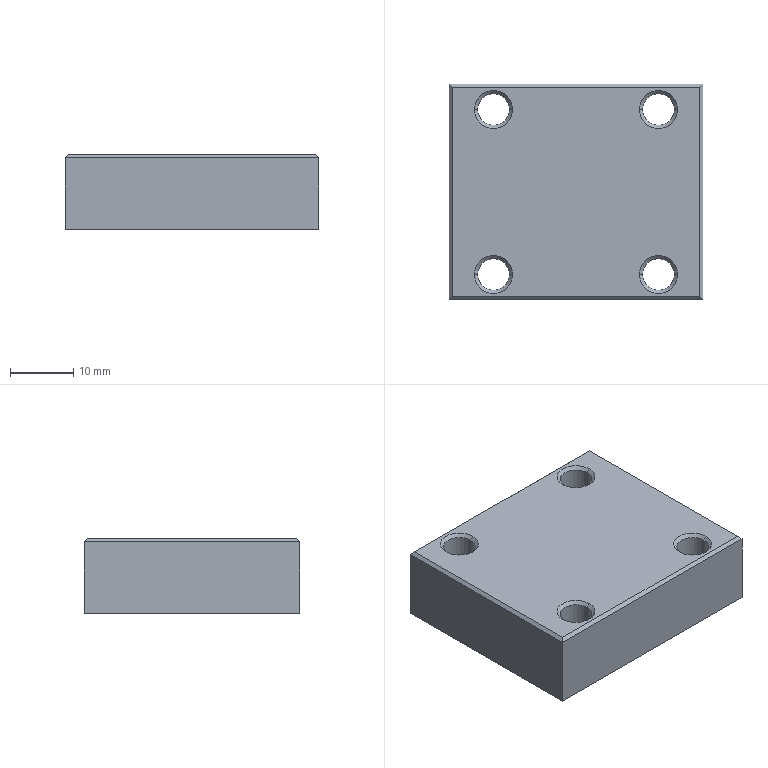Part | NX | 1 solid | 26 faces | box 40 x 34 x 11.83 mm | volume 15133 mm3 | plane 10 | cylinder 8 | cone 8 | commonest cylinder face diameters 5 x8
STEP:
#1=CARTESIAN_POINT('',(0.,0.,8.07));
#2=VERTEX_POINT('',#1);
#3=CARTESIAN_POINT('',(0.,-34.,8.07));
#4=VERTEX_POINT('',#3);
#5=CARTESIAN_POINT('',(0.,0.,8.07));
#6=DIRECTION('',(0.,-1.,0.));
#7=VECTOR('',#6,1000.);
#8=LINE('',#5,#7);
#9=EDGE_CURVE('',#2,#4,#8,.T.);
#10=ORIENTED_EDGE('',*,*,#9,.T.);
#11=CARTESIAN_POINT('',(0.5,-33.5,8.57));
#12=VERTEX_POINT('',#11);
#13=CARTESIAN_POINT('',(-8.07,-42.07,0.));
#14=DIRECTION('',(-0.5774,-0.5774,-0.5774));
#15=VECTOR('',#14,1000.);
#16=LINE('',#13,#15);
#17=EDGE_CURVE('',#12,#4,#16,.T.);
#18=ORIENTED_EDGE('',*,*,#17,.F.);
#19=CARTESIAN_POINT('',(0.5,-0.5,8.57));
#20=VERTEX_POINT('',#19);
#21=CARTESIAN_POINT('',(0.5,0.,8.57));
#22=DIRECTION('',(0.,1.,0.));
#23=VECTOR('',#22,1000.);
#24=LINE('',#21,#23);
#25=EDGE_CURVE('',#12,#20,#24,.T.);
#26=ORIENTED_EDGE('',*,*,#25,.T.);
#27=CARTESIAN_POINT('',(-8.07,8.07,0.));
#28=DIRECTION('',(-0.5774,0.5774,-0.5774));
#29=VECTOR('',#28,1000.);
#30=LINE('',#27,#29);
#31=EDGE_CURVE('',#20,#2,#30,.T.);
#32=ORIENTED_EDGE('',*,*,#31,.T.);
#33=EDGE_LOOP('',(#10,#18,#26,#32));
#34=FACE_BOUND('',#33,.T.);
#35=CARTESIAN_POINT('',(0.25,-17.,8.32));
#36=DIRECTION('',(0.7071,0.,-0.7071));
#37=DIRECTION('',(0.,-1.,0.));
#38=AXIS2_PLACEMENT_3D('',#35,#36,#37);
#39=PLANE('',#38);
#40=ADVANCED_FACE('',(#34),#39,.F.);
#41=ORIENTED_EDGE('',*,*,#9,.F.);
#42=CARTESIAN_POINT('',(0.,0.,-3.26));
#43=VERTEX_POINT('',#42);
#44=CARTESIAN_POINT('',(0.,0.,0.));
#45=DIRECTION('',(0.,0.,1.));
#46=VECTOR('',#45,1000.);
#47=LINE('',#44,#46);
#48=EDGE_CURVE('',#43,#2,#47,.T.);
#49=ORIENTED_EDGE('',*,*,#48,.F.);
#50=CARTESIAN_POINT('',(0.,-34.,-3.26));
#51=VERTEX_POINT('',#50);
#52=CARTESIAN_POINT('',(0.,0.,-3.26));
#53=DIRECTION('',(0.,-1.,0.));
#54=VECTOR('',#53,1000.);
#55=LINE('',#52,#54);
#56=EDGE_CURVE('',#43,#51,#55,.T.);
#57=ORIENTED_EDGE('',*,*,#56,.T.);
#58=CARTESIAN_POINT('',(0.,-34.,0.));
#59=DIRECTION('',(0.,0.,-1.));
#60=VECTOR('',#59,1000.);
#61=LINE('',#58,#60);
#62=EDGE_CURVE('',#4,#51,#61,.T.);
#63=ORIENTED_EDGE('',*,*,#62,.F.);
#64=EDGE_LOOP('',(#41,#49,#57,#63));
#65=FACE_BOUND('',#64,.T.);
#66=CARTESIAN_POINT('',(0.,0.,0.));
#67=DIRECTION('',(-1.,0.,0.));
#68=DIRECTION('',(0.,0.,1.));
#69=AXIS2_PLACEMENT_3D('',#66,#67,#68);
#70=PLANE('',#69);
#71=ADVANCED_FACE('',(#65),#70,.T.);
#72=CARTESIAN_POINT('',(40.,0.,8.07));
#73=VERTEX_POINT('',#72);
#74=CARTESIAN_POINT('',(0.,0.,8.07));
#75=DIRECTION('',(1.,0.,0.));
#76=VECTOR('',#75,1000.);
#77=LINE('',#74,#76);
#78=EDGE_CURVE('',#2,#73,#77,.T.);
#79=ORIENTED_EDGE('',*,*,#78,.T.);
#80=CARTESIAN_POINT('',(40.,0.,-3.26));
#81=VERTEX_POINT('',#80);
#82=CARTESIAN_POINT('',(40.,0.,0.));
#83=DIRECTION('',(0.,0.,-1.));
#84=VECTOR('',#83,1000.);
#85=LINE('',#82,#84);
#86=EDGE_CURVE('',#73,#81,#85,.T.);
#87=ORIENTED_EDGE('',*,*,#86,.T.);
#88=CARTESIAN_POINT('',(0.,0.,-3.26));
#89=DIRECTION('',(-1.,0.,0.));
#90=VECTOR('',#89,1000.);
#91=LINE('',#88,#90);
#92=EDGE_CURVE('',#81,#43,#91,.T.);
#93=ORIENTED_EDGE('',*,*,#92,.T.);
#94=ORIENTED_EDGE('',*,*,#48,.T.);
#95=EDGE_LOOP('',(#79,#87,#93,#94));
#96=FACE_BOUND('',#95,.T.);
#97=CARTESIAN_POINT('',(40.,0.,0.));
#98=DIRECTION('',(0.,1.,0.));
#99=DIRECTION('',(1.,0.,0.));
#100=AXIS2_PLACEMENT_3D('',#97,#98,#99);
#101=PLANE('',#100);
#102=ADVANCED_FACE('',(#96),#101,.T.);
#103=CARTESIAN_POINT('',(40.,-34.,8.07));
#104=VERTEX_POINT('',#103);
#105=CARTESIAN_POINT('',(40.,0.,8.07));
#106=DIRECTION('',(0.,1.,0.));
#107=VECTOR('',#106,1000.);
#108=LINE('',#105,#107);
#109=EDGE_CURVE('',#104,#73,#108,.T.);
#110=ORIENTED_EDGE('',*,*,#109,.F.);
#111=CARTESIAN_POINT('',(40.,-34.,-3.26));
#112=VERTEX_POINT('',#111);
#113=CARTESIAN_POINT('',(40.,-34.,0.));
#114=DIRECTION('',(0.,0.,1.));
#115=VECTOR('',#114,1000.);
#116=LINE('',#113,#115);
#117=EDGE_CURVE('',#112,#104,#116,.T.);
#118=ORIENTED_EDGE('',*,*,#117,.F.);
#119=CARTESIAN_POINT('',(40.,0.,-3.26));
#120=DIRECTION('',(0.,1.,0.));
#121=VECTOR('',#120,1000.);
#122=LINE('',#119,#121);
#123=EDGE_CURVE('',#112,#81,#122,.T.);
#124=ORIENTED_EDGE('',*,*,#123,.T.);
#125=ORIENTED_EDGE('',*,*,#86,.F.);
#126=EDGE_LOOP('',(#110,#118,#124,#125));
#127=FACE_BOUND('',#126,.T.);
#128=CARTESIAN_POINT('',(40.,-34.,0.));
#129=DIRECTION('',(1.,0.,0.));
#130=DIRECTION('',(0.,1.,0.));
#131=AXIS2_PLACEMENT_3D('',#128,#129,#130);
#132=PLANE('',#131);
#133=ADVANCED_FACE('',(#127),#132,.T.);
#134=CARTESIAN_POINT('',(0.,-34.,8.07));
#135=DIRECTION('',(1.,0.,0.));
#136=VECTOR('',#135,1000.);
#137=LINE('',#134,#136);
#138=EDGE_CURVE('',#4,#104,#137,.T.);
#139=ORIENTED_EDGE('',*,*,#138,.F.);
#140=ORIENTED_EDGE('',*,*,#62,.T.);
#141=CARTESIAN_POINT('',(0.,-34.,-3.26));
#142=DIRECTION('',(1.,0.,0.));
#143=VECTOR('',#142,1000.);
#144=LINE('',#141,#143);
#145=EDGE_CURVE('',#51,#112,#144,.T.);
#146=ORIENTED_EDGE('',*,*,#145,.T.);
#147=ORIENTED_EDGE('',*,*,#117,.T.);
#148=EDGE_LOOP('',(#139,#140,#146,#147));
#149=FACE_BOUND('',#148,.T.);
#150=CARTESIAN_POINT('',(0.,-34.,0.));
#151=DIRECTION('',(0.,-1.,0.));
#152=DIRECTION('',(0.,0.,-1.));
#153=AXIS2_PLACEMENT_3D('',#150,#151,#152);
#154=PLANE('',#153);
#155=ADVANCED_FACE('',(#149),#154,.T.);
#156=ORIENTED_EDGE('',*,*,#56,.F.);
#157=ORIENTED_EDGE('',*,*,#92,.F.);
#158=ORIENTED_EDGE('',*,*,#123,.F.);
#159=ORIENTED_EDGE('',*,*,#145,.F.);
#160=EDGE_LOOP('',(#156,#157,#158,#159));
#161=FACE_BOUND('',#160,.T.);
#162=CARTESIAN_POINT('',(35.5,-30.,-3.26));
#163=VERTEX_POINT('',#162);
#164=CARTESIAN_POINT('',(30.5,-30.,-3.26));
#165=VERTEX_POINT('',#164);
#166=CARTESIAN_POINT('',(33.,-30.,-3.26));
#167=DIRECTION('',(0.,0.,-1.));
#168=DIRECTION('',(-1.,0.,0.));
#169=AXIS2_PLACEMENT_3D('',#166,#167,#168);
#170=CIRCLE('',#169,2.5);
#171=EDGE_CURVE('',#163,#165,#170,.T.);
#172=ORIENTED_EDGE('',*,*,#171,.F.);
#173=CARTESIAN_POINT('',(33.,-30.,-3.26));
#174=DIRECTION('',(0.,0.,-1.));
#175=DIRECTION('',(-1.,0.,0.));
#176=AXIS2_PLACEMENT_3D('',#173,#174,#175);
#177=CIRCLE('',#176,2.5);
#178=EDGE_CURVE('',#165,#163,#177,.T.);
#179=ORIENTED_EDGE('',*,*,#178,.F.);
#180=EDGE_LOOP('',(#172,#179));
#181=FACE_BOUND('',#180,.T.);
#182=CARTESIAN_POINT('',(4.5,-30.,-3.26));
#183=VERTEX_POINT('',#182);
#184=CARTESIAN_POINT('',(9.5,-30.,-3.26));
#185=VERTEX_POINT('',#184);
#186=CARTESIAN_POINT('',(7.,-30.,-3.26));
#187=DIRECTION('',(0.,0.,-1.));
#188=DIRECTION('',(-1.,0.,0.));
#189=AXIS2_PLACEMENT_3D('',#186,#187,#188);
#190=CIRCLE('',#189,2.5);
#191=EDGE_CURVE('',#183,#185,#190,.T.);
#192=ORIENTED_EDGE('',*,*,#191,.F.);
#193=CARTESIAN_POINT('',(7.,-30.,-3.26));
#194=DIRECTION('',(0.,0.,-1.));
#195=DIRECTION('',(-1.,0.,0.));
#196=AXIS2_PLACEMENT_3D('',#193,#194,#195);
#197=CIRCLE('',#196,2.5);
#198=EDGE_CURVE('',#185,#183,#197,.T.);
#199=ORIENTED_EDGE('',*,*,#198,.F.);
#200=EDGE_LOOP('',(#192,#199));
#201=FACE_BOUND('',#200,.T.);
#202=CARTESIAN_POINT('',(30.5,-4.,-3.26));
#203=VERTEX_POINT('',#202);
#204=CARTESIAN_POINT('',(35.5,-4.,-3.26));
#205=VERTEX_POINT('',#204);
#206=CARTESIAN_POINT('',(33.,-4.,-3.26));
#207=DIRECTION('',(0.,0.,-1.));
#208=DIRECTION('',(-1.,0.,0.));
#209=AXIS2_PLACEMENT_3D('',#206,#207,#208);
#210=CIRCLE('',#209,2.5);
#211=EDGE_CURVE('',#203,#205,#210,.T.);
#212=ORIENTED_EDGE('',*,*,#211,.F.);
#213=CARTESIAN_POINT('',(33.,-4.,-3.26));
#214=DIRECTION('',(0.,0.,-1.));
#215=DIRECTION('',(-1.,0.,0.));
#216=AXIS2_PLACEMENT_3D('',#213,#214,#215);
#217=CIRCLE('',#216,2.5);
#218=EDGE_CURVE('',#205,#203,#217,.T.);
#219=ORIENTED_EDGE('',*,*,#218,.F.);
#220=EDGE_LOOP('',(#212,#219));
#221=FACE_BOUND('',#220,.T.);
#222=CARTESIAN_POINT('',(9.5,-4.,-3.26));
#223=VERTEX_POINT('',#222);
#224=CARTESIAN_POINT('',(4.5,-4.,-3.26));
#225=VERTEX_POINT('',#224);
#226=CARTESIAN_POINT('',(7.,-4.,-3.26));
#227=DIRECTION('',(0.,0.,-1.));
#228=DIRECTION('',(-1.,0.,0.));
#229=AXIS2_PLACEMENT_3D('',#226,#227,#228);
#230=CIRCLE('',#229,2.5);
#231=EDGE_CURVE('',#223,#225,#230,.T.);
#232=ORIENTED_EDGE('',*,*,#231,.F.);
#233=CARTESIAN_POINT('',(7.,-4.,-3.26));
#234=DIRECTION('',(0.,0.,-1.));
#235=DIRECTION('',(-1.,0.,0.));
#236=AXIS2_PLACEMENT_3D('',#233,#234,#235);
#237=CIRCLE('',#236,2.5);
#238=EDGE_CURVE('',#225,#223,#237,.T.);
#239=ORIENTED_EDGE('',*,*,#238,.F.);
#240=EDGE_LOOP('',(#232,#239));
#241=FACE_BOUND('',#240,.T.);
#242=CARTESIAN_POINT('',(-167.,0.,-3.26));
#243=DIRECTION('',(0.,0.,1.));
#244=DIRECTION('',(1.,0.,0.));
#245=AXIS2_PLACEMENT_3D('',#242,#243,#244);
#246=PLANE('',#245);
#247=ADVANCED_FACE('',(#161,#181,#201,#221,#241),#246,.F.);
#248=CARTESIAN_POINT('',(4.5,-4.,8.07));
#249=VERTEX_POINT('',#248);
#250=CARTESIAN_POINT('',(9.5,-4.,8.07));
#251=VERTEX_POINT('',#250);
#252=CARTESIAN_POINT('',(7.,-4.,8.07));
#253=DIRECTION('',(0.,0.,-1.));
#254=DIRECTION('',(-1.,0.,0.));
#255=AXIS2_PLACEMENT_3D('',#252,#253,#254);
#256=CIRCLE('',#255,2.5);
#257=EDGE_CURVE('',#249,#251,#256,.T.);
#258=ORIENTED_EDGE('',*,*,#257,.F.);
#259=CARTESIAN_POINT('',(4.5,-4.,10.5));
#260=DIRECTION('',(0.,0.,-1.));
#261=VECTOR('',#260,1000.);
#262=LINE('',#259,#261);
#263=EDGE_CURVE('',#225,#249,#262,.F.);
#264=ORIENTED_EDGE('',*,*,#263,.F.);
#265=ORIENTED_EDGE('',*,*,#238,.T.);
#266=CARTESIAN_POINT('',(9.5,-4.,10.5));
#267=DIRECTION('',(0.,0.,-1.));
#268=VECTOR('',#267,1000.);
#269=LINE('',#266,#268);
#270=EDGE_CURVE('',#223,#251,#269,.F.);
#271=ORIENTED_EDGE('',*,*,#270,.T.);
#272=EDGE_LOOP('',(#258,#264,#265,#271));
#273=FACE_BOUND('',#272,.T.);
#274=CARTESIAN_POINT('',(7.,-4.,10.5));
#275=DIRECTION('',(0.,0.,-1.));
#276=DIRECTION('',(-1.,0.,0.));
#277=AXIS2_PLACEMENT_3D('',#274,#275,#276);
#278=CYLINDRICAL_SURFACE('',#277,2.5);
#279=ADVANCED_FACE('',(#273),#278,.F.);
#280=ORIENTED_EDGE('',*,*,#211,.T.);
#281=CARTESIAN_POINT('',(35.5,-4.,8.07));
#282=VERTEX_POINT('',#281);
#283=CARTESIAN_POINT('',(35.5,-4.,10.5));
#284=DIRECTION('',(0.,0.,-1.));
#285=VECTOR('',#284,1000.);
#286=LINE('',#283,#285);
#287=EDGE_CURVE('',#282,#205,#286,.T.);
#288=ORIENTED_EDGE('',*,*,#287,.F.);
#289=CARTESIAN_POINT('',(30.5,-4.,8.07));
#290=VERTEX_POINT('',#289);
#291=CARTESIAN_POINT('',(33.,-4.,8.07));
#292=DIRECTION('',(0.,0.,1.));
#293=DIRECTION('',(1.,0.,0.));
#294=AXIS2_PLACEMENT_3D('',#291,#292,#293);
#295=CIRCLE('',#294,2.5);
#296=EDGE_CURVE('',#282,#290,#295,.T.);
#297=ORIENTED_EDGE('',*,*,#296,.T.);
#298=CARTESIAN_POINT('',(30.5,-4.,10.5));
#299=DIRECTION('',(0.,0.,-1.));
#300=VECTOR('',#299,1000.);
#301=LINE('',#298,#300);
#302=EDGE_CURVE('',#290,#203,#301,.T.);
#303=ORIENTED_EDGE('',*,*,#302,.T.);
#304=EDGE_LOOP('',(#280,#288,#297,#303));
#305=FACE_BOUND('',#304,.T.);
#306=CARTESIAN_POINT('',(33.,-4.,10.5));
#307=DIRECTION('',(0.,0.,-1.));
#308=DIRECTION('',(-1.,0.,0.));
#309=AXIS2_PLACEMENT_3D('',#306,#307,#308);
#310=CYLINDRICAL_SURFACE('',#309,2.5);
#311=ADVANCED_FACE('',(#305),#310,.F.);
#312=ORIENTED_EDGE('',*,*,#191,.T.);
#313=CARTESIAN_POINT('',(9.5,-30.,8.07));
#314=VERTEX_POINT('',#313);
#315=CARTESIAN_POINT('',(9.5,-30.,10.5));
#316=DIRECTION('',(0.,0.,-1.));
#317=VECTOR('',#316,1000.);
#318=LINE('',#315,#317);
#319=EDGE_CURVE('',#185,#314,#318,.F.);
#320=ORIENTED_EDGE('',*,*,#319,.T.);
#321=CARTESIAN_POINT('',(4.5,-30.,8.07));
#322=VERTEX_POINT('',#321);
#323=CARTESIAN_POINT('',(7.,-30.,8.07));
#324=DIRECTION('',(0.,0.,1.));
#325=DIRECTION('',(1.,0.,0.));
#326=AXIS2_PLACEMENT_3D('',#323,#324,#325);
#327=CIRCLE('',#326,2.5);
#328=EDGE_CURVE('',#314,#322,#327,.T.);
#329=ORIENTED_EDGE('',*,*,#328,.T.);
#330=CARTESIAN_POINT('',(4.5,-30.,10.5));
#331=DIRECTION('',(0.,0.,-1.));
#332=VECTOR('',#331,1000.);
#333=LINE('',#330,#332);
#334=EDGE_CURVE('',#183,#322,#333,.F.);
#335=ORIENTED_EDGE('',*,*,#334,.F.);
#336=EDGE_LOOP('',(#312,#320,#329,#335));
#337=FACE_BOUND('',#336,.T.);
#338=CARTESIAN_POINT('',(7.,-30.,10.5));
#339=DIRECTION('',(0.,0.,-1.));
#340=DIRECTION('',(-1.,0.,0.));
#341=AXIS2_PLACEMENT_3D('',#338,#339,#340);
#342=CYLINDRICAL_SURFACE('',#341,2.5);
#343=ADVANCED_FACE('',(#337),#342,.F.);
#344=ORIENTED_EDGE('',*,*,#171,.T.);
#345=CARTESIAN_POINT('',(30.5,-30.,8.07));
#346=VERTEX_POINT('',#345);
#347=CARTESIAN_POINT('',(30.5,-30.,10.5));
#348=DIRECTION('',(0.,0.,-1.));
#349=VECTOR('',#348,1000.);
#350=LINE('',#347,#349);
#351=EDGE_CURVE('',#165,#346,#350,.F.);
#352=ORIENTED_EDGE('',*,*,#351,.T.);
#353=CARTESIAN_POINT('',(35.5,-30.,8.07));
#354=VERTEX_POINT('',#353);
#355=CARTESIAN_POINT('',(33.,-30.,8.07));
#356=DIRECTION('',(0.,0.,-1.));
#357=DIRECTION('',(-1.,0.,0.));
#358=AXIS2_PLACEMENT_3D('',#355,#356,#357);
#359=CIRCLE('',#358,2.5);
#360=EDGE_CURVE('',#354,#346,#359,.T.);
#361=ORIENTED_EDGE('',*,*,#360,.F.);
#362=CARTESIAN_POINT('',(35.5,-30.,10.5));
#363=DIRECTION('',(0.,0.,-1.));
#364=VECTOR('',#363,1000.);
#365=LINE('',#362,#364);
#366=EDGE_CURVE('',#163,#354,#365,.F.);
#367=ORIENTED_EDGE('',*,*,#366,.F.);
#368=EDGE_LOOP('',(#344,#352,#361,#367));
#369=FACE_BOUND('',#368,.T.);
#370=CARTESIAN_POINT('',(33.,-30.,10.5));
#371=DIRECTION('',(0.,0.,-1.));
#372=DIRECTION('',(-1.,0.,0.));
#373=AXIS2_PLACEMENT_3D('',#370,#371,#372);
#374=CYLINDRICAL_SURFACE('',#373,2.5);
#375=ADVANCED_FACE('',(#369),#374,.F.);
#376=ORIENTED_EDGE('',*,*,#257,.T.);
#377=CARTESIAN_POINT('',(10.,-4.,8.57));
#378=VERTEX_POINT('',#377);
#379=CARTESIAN_POINT('',(10.,-4.,8.57));
#380=DIRECTION('',(0.7071,0.,0.7071));
#381=VECTOR('',#380,1000.);
#382=LINE('',#379,#381);
#383=EDGE_CURVE('',#251,#378,#382,.T.);
#384=ORIENTED_EDGE('',*,*,#383,.T.);
#385=CARTESIAN_POINT('',(4.,-4.,8.57));
#386=VERTEX_POINT('',#385);
#387=CARTESIAN_POINT('',(7.,-4.,8.57));
#388=DIRECTION('',(0.,0.,1.));
#389=DIRECTION('',(1.,0.,0.));
#390=AXIS2_PLACEMENT_3D('',#387,#388,#389);
#391=CIRCLE('',#390,3.);
#392=EDGE_CURVE('',#378,#386,#391,.T.);
#393=ORIENTED_EDGE('',*,*,#392,.T.);
#394=CARTESIAN_POINT('',(4.,-4.,8.57));
#395=DIRECTION('',(-0.7071,0.,0.7071));
#396=VECTOR('',#395,1000.);
#397=LINE('',#394,#396);
#398=EDGE_CURVE('',#249,#386,#397,.T.);
#399=ORIENTED_EDGE('',*,*,#398,.F.);
#400=EDGE_LOOP('',(#376,#384,#393,#399));
#401=FACE_BOUND('',#400,.T.);
#402=CARTESIAN_POINT('',(7.,-4.,8.57));
#403=DIRECTION('',(0.,0.,1.));
#404=DIRECTION('',(1.,0.,0.));
#405=AXIS2_PLACEMENT_3D('',#402,#403,#404);
#406=CONICAL_SURFACE('',#405,3.,0.7854);
#407=ADVANCED_FACE('',(#401),#406,.F.);
#408=CARTESIAN_POINT('',(10.,-30.,8.57));
#409=VERTEX_POINT('',#408);
#410=CARTESIAN_POINT('',(4.,-30.,8.57));
#411=VERTEX_POINT('',#410);
#412=CARTESIAN_POINT('',(7.,-30.,8.57));
#413=DIRECTION('',(0.,0.,1.));
#414=DIRECTION('',(1.,0.,0.));
#415=AXIS2_PLACEMENT_3D('',#412,#413,#414);
#416=CIRCLE('',#415,3.);
#417=EDGE_CURVE('',#409,#411,#416,.T.);
#418=ORIENTED_EDGE('',*,*,#417,.T.);
#419=CARTESIAN_POINT('',(4.,-30.,8.57));
#420=DIRECTION('',(-0.7071,0.,0.7071));
#421=VECTOR('',#420,1000.);
#422=LINE('',#419,#421);
#423=EDGE_CURVE('',#322,#411,#422,.T.);
#424=ORIENTED_EDGE('',*,*,#423,.F.);
#425=ORIENTED_EDGE('',*,*,#328,.F.);
#426=CARTESIAN_POINT('',(10.,-30.,8.57));
#427=DIRECTION('',(0.7071,0.,0.7071));
#428=VECTOR('',#427,1000.);
#429=LINE('',#426,#428);
#430=EDGE_CURVE('',#314,#409,#429,.T.);
#431=ORIENTED_EDGE('',*,*,#430,.T.);
#432=EDGE_LOOP('',(#418,#424,#425,#431));
#433=FACE_BOUND('',#432,.T.);
#434=CARTESIAN_POINT('',(7.,-30.,8.57));
#435=DIRECTION('',(0.,0.,1.));
#436=DIRECTION('',(1.,0.,0.));
#437=AXIS2_PLACEMENT_3D('',#434,#435,#436);
#438=CONICAL_SURFACE('',#437,3.,0.7854);
#439=ADVANCED_FACE('',(#433),#438,.F.);
#440=CARTESIAN_POINT('',(33.,-30.,8.07));
#441=DIRECTION('',(0.,0.,-1.));
#442=DIRECTION('',(-1.,0.,0.));
#443=AXIS2_PLACEMENT_3D('',#440,#441,#442);
#444=CIRCLE('',#443,2.5);
#445=EDGE_CURVE('',#346,#354,#444,.T.);
#446=ORIENTED_EDGE('',*,*,#445,.T.);
#447=CARTESIAN_POINT('',(36.,-30.,8.57));
#448=VERTEX_POINT('',#447);
#449=CARTESIAN_POINT('',(36.,-30.,8.57));
#450=DIRECTION('',(0.7071,0.,0.7071));
#451=VECTOR('',#450,1000.);
#452=LINE('',#449,#451);
#453=EDGE_CURVE('',#354,#448,#452,.T.);
#454=ORIENTED_EDGE('',*,*,#453,.T.);
#455=CARTESIAN_POINT('',(30.,-30.,8.57));
#456=VERTEX_POINT('',#455);
#457=CARTESIAN_POINT('',(33.,-30.,8.57));
#458=DIRECTION('',(0.,0.,1.));
#459=DIRECTION('',(1.,0.,0.));
#460=AXIS2_PLACEMENT_3D('',#457,#458,#459);
#461=CIRCLE('',#460,3.);
#462=EDGE_CURVE('',#448,#456,#461,.T.);
#463=ORIENTED_EDGE('',*,*,#462,.T.);
#464=CARTESIAN_POINT('',(30.,-30.,8.57));
#465=DIRECTION('',(-0.7071,0.,0.7071));
#466=VECTOR('',#465,1000.);
#467=LINE('',#464,#466);
#468=EDGE_CURVE('',#346,#456,#467,.T.);
#469=ORIENTED_EDGE('',*,*,#468,.F.);
#470=EDGE_LOOP('',(#446,#454,#463,#469));
#471=FACE_BOUND('',#470,.T.);
#472=CARTESIAN_POINT('',(33.,-30.,8.57));
#473=DIRECTION('',(0.,0.,1.));
#474=DIRECTION('',(1.,0.,0.));
#475=AXIS2_PLACEMENT_3D('',#472,#473,#474);
#476=CONICAL_SURFACE('',#475,3.,0.7854);
#477=ADVANCED_FACE('',(#471),#476,.F.);
#478=CARTESIAN_POINT('',(36.,-4.,8.57));
#479=VERTEX_POINT('',#478);
#480=CARTESIAN_POINT('',(30.,-4.,8.57));
#481=VERTEX_POINT('',#480);
#482=CARTESIAN_POINT('',(33.,-4.,8.57));
#483=DIRECTION('',(0.,0.,1.));
#484=DIRECTION('',(1.,0.,0.));
#485=AXIS2_PLACEMENT_3D('',#482,#483,#484);
#486=CIRCLE('',#485,3.);
#487=EDGE_CURVE('',#479,#481,#486,.T.);
#488=ORIENTED_EDGE('',*,*,#487,.T.);
#489=CARTESIAN_POINT('',(30.,-4.,8.57));
#490=DIRECTION('',(-0.7071,0.,0.7071));
#491=VECTOR('',#490,1000.);
#492=LINE('',#489,#491);
#493=EDGE_CURVE('',#481,#290,#492,.F.);
#494=ORIENTED_EDGE('',*,*,#493,.T.);
#495=ORIENTED_EDGE('',*,*,#296,.F.);
#496=CARTESIAN_POINT('',(36.,-4.,8.57));
#497=DIRECTION('',(0.7071,0.,0.7071));
#498=VECTOR('',#497,1000.);
#499=LINE('',#496,#498);
#500=EDGE_CURVE('',#479,#282,#499,.F.);
#501=ORIENTED_EDGE('',*,*,#500,.F.);
#502=EDGE_LOOP('',(#488,#494,#495,#501));
#503=FACE_BOUND('',#502,.T.);
#504=CARTESIAN_POINT('',(33.,-4.,8.57));
#505=DIRECTION('',(0.,0.,1.));
#506=DIRECTION('',(1.,0.,0.));
#507=AXIS2_PLACEMENT_3D('',#504,#505,#506);
#508=CONICAL_SURFACE('',#507,3.,0.7854);
#509=ADVANCED_FACE('',(#503),#508,.F.);
#510=ORIENTED_EDGE('',*,*,#138,.T.);
#511=CARTESIAN_POINT('',(39.5,-33.5,8.57));
#512=VERTEX_POINT('',#511);
#513=CARTESIAN_POINT('',(48.07,-42.07,0.));
#514=DIRECTION('',(-0.5774,0.5774,0.5774));
#515=VECTOR('',#514,1000.);
#516=LINE('',#513,#515);
#517=EDGE_CURVE('',#104,#512,#516,.T.);
#518=ORIENTED_EDGE('',*,*,#517,.T.);
#519=CARTESIAN_POINT('',(0.,-33.5,8.57));
#520=DIRECTION('',(1.,0.,0.));
#521=VECTOR('',#520,1000.);
#522=LINE('',#519,#521);
#523=EDGE_CURVE('',#12,#512,#522,.T.);
#524=ORIENTED_EDGE('',*,*,#523,.F.);
#525=ORIENTED_EDGE('',*,*,#17,.T.);
#526=EDGE_LOOP('',(#510,#518,#524,#525));
#527=FACE_BOUND('',#526,.T.);
#528=CARTESIAN_POINT('',(20.,-33.75,8.32));
#529=DIRECTION('',(0.,0.7071,-0.7071));
#530=DIRECTION('',(-1.,0.,0.));
#531=AXIS2_PLACEMENT_3D('',#528,#529,#530);
#532=PLANE('',#531);
#533=ADVANCED_FACE('',(#527),#532,.F.);
#534=ORIENTED_EDGE('',*,*,#109,.T.);
#535=CARTESIAN_POINT('',(39.5,-0.5,8.57));
#536=VERTEX_POINT('',#535);
#537=CARTESIAN_POINT('',(48.07,8.07,0.));
#538=DIRECTION('',(-0.5774,-0.5774,0.5774));
#539=VECTOR('',#538,1000.);
#540=LINE('',#537,#539);
#541=EDGE_CURVE('',#73,#536,#540,.T.);
#542=ORIENTED_EDGE('',*,*,#541,.T.);
#543=CARTESIAN_POINT('',(39.5,0.,8.57));
#544=DIRECTION('',(0.,-1.,0.));
#545=VECTOR('',#544,1000.);
#546=LINE('',#543,#545);
#547=EDGE_CURVE('',#536,#512,#546,.T.);
#548=ORIENTED_EDGE('',*,*,#547,.T.);
#549=ORIENTED_EDGE('',*,*,#517,.F.);
#550=EDGE_LOOP('',(#534,#542,#548,#549));
#551=FACE_BOUND('',#550,.T.);
#552=CARTESIAN_POINT('',(39.75,-17.,8.32));
#553=DIRECTION('',(0.7071,0.,0.7071));
#554=DIRECTION('',(0.,-1.,0.));
#555=AXIS2_PLACEMENT_3D('',#552,#553,#554);
#556=PLANE('',#555);
#557=ADVANCED_FACE('',(#551),#556,.T.);
#558=ORIENTED_EDGE('',*,*,#78,.F.);
#559=ORIENTED_EDGE('',*,*,#31,.F.);
#560=CARTESIAN_POINT('',(0.,-0.5,8.57));
#561=DIRECTION('',(1.,0.,0.));
#562=VECTOR('',#561,1000.);
#563=LINE('',#560,#562);
#564=EDGE_CURVE('',#20,#536,#563,.T.);
#565=ORIENTED_EDGE('',*,*,#564,.T.);
#566=ORIENTED_EDGE('',*,*,#541,.F.);
#567=EDGE_LOOP('',(#558,#559,#565,#566));
#568=FACE_BOUND('',#567,.T.);
#569=CARTESIAN_POINT('',(20.,-0.25,8.32));
#570=DIRECTION('',(0.,0.7071,0.7071));
#571=DIRECTION('',(1.,0.,0.));
#572=AXIS2_PLACEMENT_3D('',#569,#570,#571);
#573=PLANE('',#572);
#574=ADVANCED_FACE('',(#568),#573,.T.);
#575=ORIENTED_EDGE('',*,*,#25,.F.);
#576=ORIENTED_EDGE('',*,*,#523,.T.);
#577=ORIENTED_EDGE('',*,*,#547,.F.);
#578=ORIENTED_EDGE('',*,*,#564,.F.);
#579=EDGE_LOOP('',(#575,#576,#577,#578));
#580=FACE_BOUND('',#579,.T.);
#581=ORIENTED_EDGE('',*,*,#392,.F.);
#582=CARTESIAN_POINT('',(7.,-4.,8.57));
#583=DIRECTION('',(0.,0.,1.));
#584=DIRECTION('',(1.,0.,0.));
#585=AXIS2_PLACEMENT_3D('',#582,#583,#584);
#586=CIRCLE('',#585,3.);
#587=EDGE_CURVE('',#386,#378,#586,.T.);
#588=ORIENTED_EDGE('',*,*,#587,.F.);
#589=EDGE_LOOP('',(#581,#588));
#590=FACE_BOUND('',#589,.T.);
#591=ORIENTED_EDGE('',*,*,#462,.F.);
#592=CARTESIAN_POINT('',(33.,-30.,8.57));
#593=DIRECTION('',(0.,0.,1.));
#594=DIRECTION('',(1.,0.,0.));
#595=AXIS2_PLACEMENT_3D('',#592,#593,#594);
#596=CIRCLE('',#595,3.);
#597=EDGE_CURVE('',#456,#448,#596,.T.);
#598=ORIENTED_EDGE('',*,*,#597,.F.);
#599=EDGE_LOOP('',(#591,#598));
#600=FACE_BOUND('',#599,.T.);
#601=ORIENTED_EDGE('',*,*,#487,.F.);
#602=CARTESIAN_POINT('',(33.,-4.,8.57));
#603=DIRECTION('',(0.,0.,1.));
#604=DIRECTION('',(1.,0.,0.));
#605=AXIS2_PLACEMENT_3D('',#602,#603,#604);
#606=CIRCLE('',#605,3.);
#607=EDGE_CURVE('',#481,#479,#606,.T.);
#608=ORIENTED_EDGE('',*,*,#607,.F.);
#609=EDGE_LOOP('',(#601,#608));
#610=FACE_BOUND('',#609,.T.);
#611=ORIENTED_EDGE('',*,*,#417,.F.);
#612=CARTESIAN_POINT('',(7.,-30.,8.57));
#613=DIRECTION('',(0.,0.,1.));
#614=DIRECTION('',(1.,0.,0.));
#615=AXIS2_PLACEMENT_3D('',#612,#613,#614);
#616=CIRCLE('',#615,3.);
#617=EDGE_CURVE('',#411,#409,#616,.T.);
#618=ORIENTED_EDGE('',*,*,#617,.F.);
#619=EDGE_LOOP('',(#611,#618));
#620=FACE_BOUND('',#619,.T.);
#621=CARTESIAN_POINT('',(0.,0.,8.57));
#622=DIRECTION('',(0.,0.,1.));
#623=DIRECTION('',(1.,0.,0.));
#624=AXIS2_PLACEMENT_3D('',#621,#622,#623);
#625=PLANE('',#624);
#626=ADVANCED_FACE('',(#580,#590,#600,#610,#620),#625,.T.);
#627=ORIENTED_EDGE('',*,*,#445,.F.);
#628=ORIENTED_EDGE('',*,*,#351,.F.);
#629=ORIENTED_EDGE('',*,*,#178,.T.);
#630=ORIENTED_EDGE('',*,*,#366,.T.);
#631=EDGE_LOOP('',(#627,#628,#629,#630));
#632=FACE_BOUND('',#631,.T.);
#633=CARTESIAN_POINT('',(33.,-30.,10.5));
#634=DIRECTION('',(0.,0.,-1.));
#635=DIRECTION('',(-1.,0.,0.));
#636=AXIS2_PLACEMENT_3D('',#633,#634,#635);
#637=CYLINDRICAL_SURFACE('',#636,2.5);
#638=ADVANCED_FACE('',(#632),#637,.F.);
#639=CARTESIAN_POINT('',(33.,-4.,8.07));
#640=DIRECTION('',(0.,0.,1.));
#641=DIRECTION('',(1.,0.,0.));
#642=AXIS2_PLACEMENT_3D('',#639,#640,#641);
#643=CIRCLE('',#642,2.5);
#644=EDGE_CURVE('',#290,#282,#643,.T.);
#645=ORIENTED_EDGE('',*,*,#644,.F.);
#646=ORIENTED_EDGE('',*,*,#493,.F.);
#647=ORIENTED_EDGE('',*,*,#607,.T.);
#648=ORIENTED_EDGE('',*,*,#500,.T.);
#649=EDGE_LOOP('',(#645,#646,#647,#648));
#650=FACE_BOUND('',#649,.T.);
#651=CARTESIAN_POINT('',(33.,-4.,8.57));
#652=DIRECTION('',(0.,0.,1.));
#653=DIRECTION('',(1.,0.,0.));
#654=AXIS2_PLACEMENT_3D('',#651,#652,#653);
#655=CONICAL_SURFACE('',#654,3.,0.7854);
#656=ADVANCED_FACE('',(#650),#655,.F.);
#657=ORIENTED_EDGE('',*,*,#231,.T.);
#658=ORIENTED_EDGE('',*,*,#263,.T.);
#659=CARTESIAN_POINT('',(7.,-4.,8.07));
#660=DIRECTION('',(0.,0.,-1.));
#661=DIRECTION('',(-1.,0.,0.));
#662=AXIS2_PLACEMENT_3D('',#659,#660,#661);
#663=CIRCLE('',#662,2.5);
#664=EDGE_CURVE('',#251,#249,#663,.T.);
#665=ORIENTED_EDGE('',*,*,#664,.F.);
#666=ORIENTED_EDGE('',*,*,#270,.F.);
#667=EDGE_LOOP('',(#657,#658,#665,#666));
#668=FACE_BOUND('',#667,.T.);
#669=CARTESIAN_POINT('',(7.,-4.,10.5));
#670=DIRECTION('',(0.,0.,-1.));
#671=DIRECTION('',(-1.,0.,0.));
#672=AXIS2_PLACEMENT_3D('',#669,#670,#671);
#673=CYLINDRICAL_SURFACE('',#672,2.5);
#674=ADVANCED_FACE('',(#668),#673,.F.);
#675=ORIENTED_EDGE('',*,*,#383,.F.);
#676=ORIENTED_EDGE('',*,*,#664,.T.);
#677=ORIENTED_EDGE('',*,*,#398,.T.);
#678=ORIENTED_EDGE('',*,*,#587,.T.);
#679=EDGE_LOOP('',(#675,#676,#677,#678));
#680=FACE_BOUND('',#679,.T.);
#681=CARTESIAN_POINT('',(7.,-4.,8.57));
#682=DIRECTION('',(0.,0.,1.));
#683=DIRECTION('',(1.,0.,0.));
#684=AXIS2_PLACEMENT_3D('',#681,#682,#683);
#685=CONICAL_SURFACE('',#684,3.,0.7854);
#686=ADVANCED_FACE('',(#680),#685,.F.);
#687=ORIENTED_EDGE('',*,*,#644,.T.);
#688=ORIENTED_EDGE('',*,*,#287,.T.);
#689=ORIENTED_EDGE('',*,*,#218,.T.);
#690=ORIENTED_EDGE('',*,*,#302,.F.);
#691=EDGE_LOOP('',(#687,#688,#689,#690));
#692=FACE_BOUND('',#691,.T.);
#693=CARTESIAN_POINT('',(33.,-4.,10.5));
#694=DIRECTION('',(0.,0.,-1.));
#695=DIRECTION('',(-1.,0.,0.));
#696=AXIS2_PLACEMENT_3D('',#693,#694,#695);
#697=CYLINDRICAL_SURFACE('',#696,2.5);
#698=ADVANCED_FACE('',(#692),#697,.F.);
#699=ORIENTED_EDGE('',*,*,#430,.F.);
#700=CARTESIAN_POINT('',(7.,-30.,8.07));
#701=DIRECTION('',(0.,0.,1.));
#702=DIRECTION('',(1.,0.,0.));
#703=AXIS2_PLACEMENT_3D('',#700,#701,#702);
#704=CIRCLE('',#703,2.5);
#705=EDGE_CURVE('',#322,#314,#704,.T.);
#706=ORIENTED_EDGE('',*,*,#705,.F.);
#707=ORIENTED_EDGE('',*,*,#423,.T.);
#708=ORIENTED_EDGE('',*,*,#617,.T.);
#709=EDGE_LOOP('',(#699,#706,#707,#708));
#710=FACE_BOUND('',#709,.T.);
#711=CARTESIAN_POINT('',(7.,-30.,8.57));
#712=DIRECTION('',(0.,0.,1.));
#713=DIRECTION('',(1.,0.,0.));
#714=AXIS2_PLACEMENT_3D('',#711,#712,#713);
#715=CONICAL_SURFACE('',#714,3.,0.7854);
#716=ADVANCED_FACE('',(#710),#715,.F.);
#717=ORIENTED_EDGE('',*,*,#334,.T.);
#718=ORIENTED_EDGE('',*,*,#705,.T.);
#719=ORIENTED_EDGE('',*,*,#319,.F.);
#720=ORIENTED_EDGE('',*,*,#198,.T.);
#721=EDGE_LOOP('',(#717,#718,#719,#720));
#722=FACE_BOUND('',#721,.T.);
#723=CARTESIAN_POINT('',(7.,-30.,10.5));
#724=DIRECTION('',(0.,0.,-1.));
#725=DIRECTION('',(-1.,0.,0.));
#726=AXIS2_PLACEMENT_3D('',#723,#724,#725);
#727=CYLINDRICAL_SURFACE('',#726,2.5);
#728=ADVANCED_FACE('',(#722),#727,.F.);
#729=ORIENTED_EDGE('',*,*,#453,.F.);
#730=ORIENTED_EDGE('',*,*,#360,.T.);
#731=ORIENTED_EDGE('',*,*,#468,.T.);
#732=ORIENTED_EDGE('',*,*,#597,.T.);
#733=EDGE_LOOP('',(#729,#730,#731,#732));
#734=FACE_BOUND('',#733,.T.);
#735=CARTESIAN_POINT('',(33.,-30.,8.57));
#736=DIRECTION('',(0.,0.,1.));
#737=DIRECTION('',(1.,0.,0.));
#738=AXIS2_PLACEMENT_3D('',#735,#736,#737);
#739=CONICAL_SURFACE('',#738,3.,0.7854);
#740=ADVANCED_FACE('',(#734),#739,.F.);
#741=CLOSED_SHELL('',(#40,#71,#102,#133,#155,#247,#279,#311,#343,#375,#407,#439,#477,#509,#533,#557,#574,#626,#638,#656,#674,#686,#698,#716,#728,#740));
#742=MANIFOLD_SOLID_BREP('',#741);
#743=(LENGTH_UNIT()NAMED_UNIT(*)SI_UNIT(.MILLI.,.METRE.));
#744=UNCERTAINTY_MEASURE_WITH_UNIT(LENGTH_MEASURE(0.00001),#743,'','');
#745=(NAMED_UNIT(*)PLANE_ANGLE_UNIT()SI_UNIT($,.RADIAN.));
#746=(NAMED_UNIT(*)SI_UNIT($,.STERADIAN.)SOLID_ANGLE_UNIT());
#747=(GEOMETRIC_REPRESENTATION_CONTEXT(3)GLOBAL_UNCERTAINTY_ASSIGNED_CONTEXT((#744))GLOBAL_UNIT_ASSIGNED_CONTEXT((#743,#745,#746))REPRESENTATION_CONTEXT('',''));
#748=ADVANCED_BREP_SHAPE_REPRESENTATION('',(#742),#747);